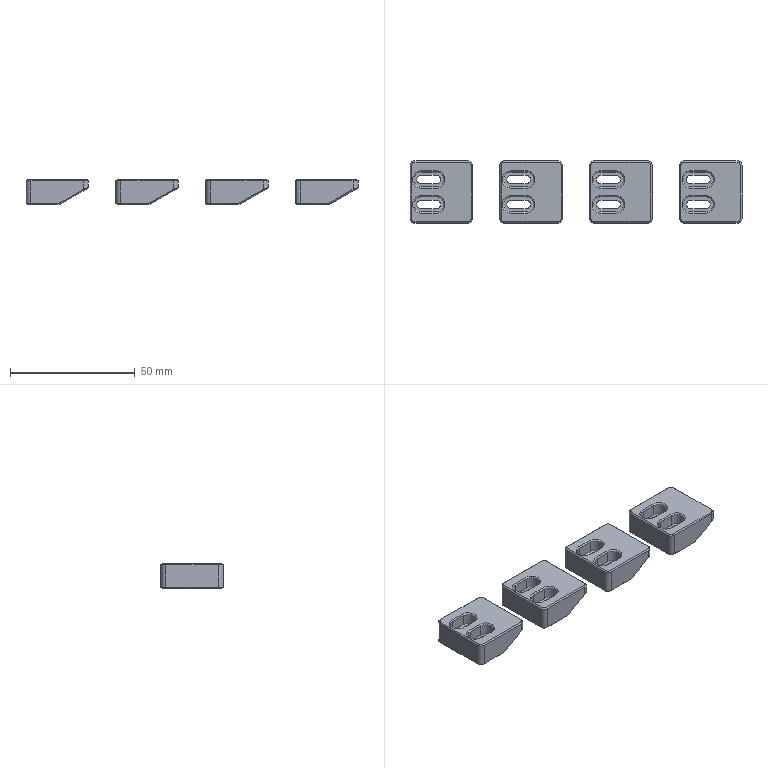NC program | NX | posted with a generic post | part box 133 x 25 x 10 mm
Lines 1 to 50 of 3677:
N10 G17 G21 G94 G90
(FLOOR_WALL_COPY , TOOL : D80)
N12 T19 M6
N14 G54
N16 G17 G0 G90 X109.5 Y0. S6500 M3
N18 G43 Z30. H19
N20 Z7.
N22 G94 G1 Z4. F1500.
N24 X106.5
N26 X-106.5
N28 X-109.5
N30 Z7.
N32 G0 Z30.
N34 X109.5
N36 Z6.
N38 G1 Z3.
N40 X106.5
N42 X-106.5
N44 X-109.5
N46 Z6.
N48 G0 Z30.
N50 X109.5
N52 Z5.
N54 G1 Z2.
N56 X106.5
N58 X-106.5
N60 X-109.5
N62 Z5.
N64 G0 Z30.
N66 X109.5
N68 Z4.
N70 G1 Z1.
N72 X106.5
N74 X-106.5
N76 X-109.5
N78 Z4.
N80 G0 Z30.
N82 X109.5
N84 Z3.
N86 G1 Z0.
N88 X106.5
N90 X-106.5
N92 X-109.5
N94 Z3.
N96 G0 Z30.
N98 M5